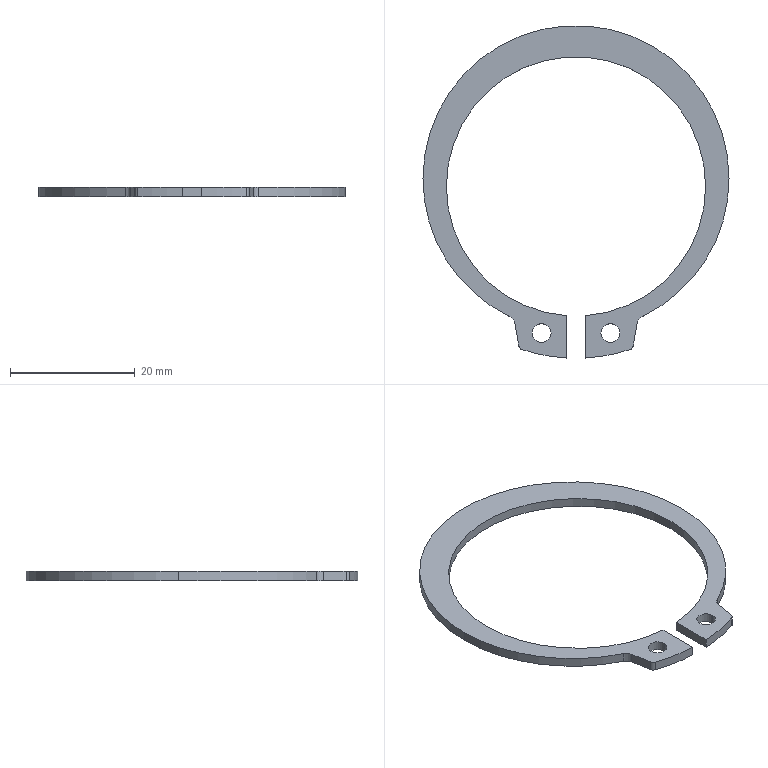Part | SolidWorks | features BaseBody 1 | 1 solid | 22 faces | box 49 x 53.209 x 1.5 mm | volume 871.359 mm3 | cylinder 16 | plane 6 | commonest cylinder face diameters 3 x6 41.5 x3 49 x3 1.4 x2 55 x2
STEP:
#1=CARTESIAN_POINT('',(4.,-24.714,-1.5));
#2=VERTEX_POINT('',#1);
#3=CARTESIAN_POINT('',(7.,-24.714,-1.5));
#4=VERTEX_POINT('',#3);
#5=CARTESIAN_POINT('',(5.5,-24.714,-1.5));
#6=DIRECTION('',(0.,0.,1.));
#7=DIRECTION('',(-1.,0.,0.));
#8=AXIS2_PLACEMENT_3D('',#5,#6,#7);
#9=CIRCLE('',#8,1.5);
#10=EDGE_CURVE('',#2,#4,#9,.T.);
#11=ORIENTED_EDGE('',*,*,#10,.F.);
#12=CARTESIAN_POINT('',(4.,-24.714,0.));
#13=VERTEX_POINT('',#12);
#14=CARTESIAN_POINT('',(4.,-24.714,-1.5));
#15=DIRECTION('',(0.,0.,1.));
#16=VECTOR('',#15,1000.);
#17=LINE('',#14,#16);
#18=EDGE_CURVE('',#2,#13,#17,.T.);
#19=ORIENTED_EDGE('',*,*,#18,.T.);
#20=CARTESIAN_POINT('',(7.,-24.714,0.));
#21=VERTEX_POINT('',#20);
#22=CARTESIAN_POINT('',(5.5,-24.714,0.));
#23=DIRECTION('',(0.,0.,1.));
#24=DIRECTION('',(-1.,0.,0.));
#25=AXIS2_PLACEMENT_3D('',#22,#23,#24);
#26=CIRCLE('',#25,1.5);
#27=EDGE_CURVE('',#13,#21,#26,.T.);
#28=ORIENTED_EDGE('',*,*,#27,.T.);
#29=CARTESIAN_POINT('',(7.,-24.714,-1.5));
#30=DIRECTION('',(0.,0.,1.));
#31=VECTOR('',#30,1000.);
#32=LINE('',#29,#31);
#33=EDGE_CURVE('',#4,#21,#32,.T.);
#34=ORIENTED_EDGE('',*,*,#33,.F.);
#35=EDGE_LOOP('',(#11,#19,#28,#34));
#36=FACE_OUTER_BOUND('',#35,.T.);
#37=CARTESIAN_POINT('',(5.5,-24.714,-1.5));
#38=DIRECTION('',(0.,0.,1.));
#39=DIRECTION('',(1.,0.,0.));
#40=AXIS2_PLACEMENT_3D('',#37,#38,#39);
#41=CYLINDRICAL_SURFACE('',#40,1.5);
#42=ADVANCED_FACE('',(#36),#41,.F.);
#43=CARTESIAN_POINT('',(-7.,-24.714,-1.5));
#44=VERTEX_POINT('',#43);
#45=CARTESIAN_POINT('',(-4.,-24.714,-1.5));
#46=VERTEX_POINT('',#45);
#47=CARTESIAN_POINT('',(-5.5,-24.714,-1.5));
#48=DIRECTION('',(0.,0.,1.));
#49=DIRECTION('',(1.,0.,0.));
#50=AXIS2_PLACEMENT_3D('',#47,#48,#49);
#51=CIRCLE('',#50,1.5);
#52=EDGE_CURVE('',#44,#46,#51,.T.);
#53=ORIENTED_EDGE('',*,*,#52,.F.);
#54=CARTESIAN_POINT('',(-7.,-24.714,0.));
#55=VERTEX_POINT('',#54);
#56=CARTESIAN_POINT('',(-7.,-24.714,-1.5));
#57=DIRECTION('',(0.,0.,1.));
#58=VECTOR('',#57,1000.);
#59=LINE('',#56,#58);
#60=EDGE_CURVE('',#44,#55,#59,.T.);
#61=ORIENTED_EDGE('',*,*,#60,.T.);
#62=CARTESIAN_POINT('',(-4.,-24.714,0.));
#63=VERTEX_POINT('',#62);
#64=CARTESIAN_POINT('',(-5.5,-24.714,0.));
#65=DIRECTION('',(0.,0.,1.));
#66=DIRECTION('',(1.,0.,0.));
#67=AXIS2_PLACEMENT_3D('',#64,#65,#66);
#68=CIRCLE('',#67,1.5);
#69=EDGE_CURVE('',#55,#63,#68,.T.);
#70=ORIENTED_EDGE('',*,*,#69,.T.);
#71=CARTESIAN_POINT('',(-4.,-24.714,-1.5));
#72=DIRECTION('',(0.,0.,1.));
#73=VECTOR('',#72,1000.);
#74=LINE('',#71,#73);
#75=EDGE_CURVE('',#46,#63,#74,.T.);
#76=ORIENTED_EDGE('',*,*,#75,.F.);
#77=EDGE_LOOP('',(#53,#61,#70,#76));
#78=FACE_OUTER_BOUND('',#77,.T.);
#79=CARTESIAN_POINT('',(-5.5,-24.714,-1.5));
#80=DIRECTION('',(0.,0.,1.));
#81=DIRECTION('',(1.,0.,0.));
#82=AXIS2_PLACEMENT_3D('',#79,#80,#81);
#83=CYLINDRICAL_SURFACE('',#82,1.5);
#84=ADVANCED_FACE('',(#78),#83,.F.);
#85=CARTESIAN_POINT('',(24.5,0.,-1.5));
#86=VERTEX_POINT('',#85);
#87=CARTESIAN_POINT('',(-24.5,0.,-1.5));
#88=VERTEX_POINT('',#87);
#89=CARTESIAN_POINT('',(0.,0.,-1.5));
#90=DIRECTION('',(0.,0.,1.));
#91=DIRECTION('',(1.,0.,0.));
#92=AXIS2_PLACEMENT_3D('',#89,#90,#91);
#93=CIRCLE('',#92,24.5);
#94=EDGE_CURVE('',#86,#88,#93,.T.);
#95=ORIENTED_EDGE('',*,*,#94,.T.);
#96=CARTESIAN_POINT('',(-24.5,0.,0.));
#97=VERTEX_POINT('',#96);
#98=CARTESIAN_POINT('',(-24.5,0.,-1.5));
#99=DIRECTION('',(0.,0.,1.));
#100=VECTOR('',#99,1000.);
#101=LINE('',#98,#100);
#102=EDGE_CURVE('',#88,#97,#101,.T.);
#103=ORIENTED_EDGE('',*,*,#102,.T.);
#104=CARTESIAN_POINT('',(24.5,0.,0.));
#105=VERTEX_POINT('',#104);
#106=CARTESIAN_POINT('',(0.,0.,0.));
#107=DIRECTION('',(0.,0.,1.));
#108=DIRECTION('',(1.,0.,0.));
#109=AXIS2_PLACEMENT_3D('',#106,#107,#108);
#110=CIRCLE('',#109,24.5);
#111=EDGE_CURVE('',#105,#97,#110,.T.);
#112=ORIENTED_EDGE('',*,*,#111,.F.);
#113=CARTESIAN_POINT('',(24.5,0.,-1.5));
#114=DIRECTION('',(0.,0.,1.));
#115=VECTOR('',#114,1000.);
#116=LINE('',#113,#115);
#117=EDGE_CURVE('',#86,#105,#116,.T.);
#118=ORIENTED_EDGE('',*,*,#117,.F.);
#119=EDGE_LOOP('',(#95,#103,#112,#118));
#120=FACE_OUTER_BOUND('',#119,.T.);
#121=CARTESIAN_POINT('',(0.,0.,-1.5));
#122=DIRECTION('',(0.,0.,1.));
#123=DIRECTION('',(1.,0.,0.));
#124=AXIS2_PLACEMENT_3D('',#121,#122,#123);
#125=CYLINDRICAL_SURFACE('',#124,24.5);
#126=ADVANCED_FACE('',(#120),#125,.T.);
#127=CARTESIAN_POINT('',(10.615,-22.081,-1.5));
#128=VERTEX_POINT('',#127);
#129=CARTESIAN_POINT('',(0.,0.,-1.5));
#130=DIRECTION('',(0.,0.,1.));
#131=DIRECTION('',(1.,0.,0.));
#132=AXIS2_PLACEMENT_3D('',#129,#130,#131);
#133=CIRCLE('',#132,24.5);
#134=EDGE_CURVE('',#128,#86,#133,.T.);
#135=ORIENTED_EDGE('',*,*,#134,.T.);
#136=ORIENTED_EDGE('',*,*,#117,.T.);
#137=CARTESIAN_POINT('',(10.615,-22.081,0.));
#138=VERTEX_POINT('',#137);
#139=CARTESIAN_POINT('',(0.,0.,0.));
#140=DIRECTION('',(0.,0.,1.));
#141=DIRECTION('',(1.,0.,0.));
#142=AXIS2_PLACEMENT_3D('',#139,#140,#141);
#143=CIRCLE('',#142,24.5);
#144=EDGE_CURVE('',#138,#105,#143,.T.);
#145=ORIENTED_EDGE('',*,*,#144,.F.);
#146=CARTESIAN_POINT('',(10.615,-22.081,-1.5));
#147=DIRECTION('',(0.,0.,-1.));
#148=VECTOR('',#147,1000.);
#149=LINE('',#146,#148);
#150=EDGE_CURVE('',#138,#128,#149,.T.);
#151=ORIENTED_EDGE('',*,*,#150,.T.);
#152=EDGE_LOOP('',(#135,#136,#145,#151));
#153=FACE_OUTER_BOUND('',#152,.T.);
#154=CARTESIAN_POINT('',(0.,0.,-1.5));
#155=DIRECTION('',(0.,0.,1.));
#156=DIRECTION('',(1.,0.,0.));
#157=AXIS2_PLACEMENT_3D('',#154,#155,#156);
#158=CYLINDRICAL_SURFACE('',#157,24.5);
#159=ADVANCED_FACE('',(#153),#158,.T.);
#160=CARTESIAN_POINT('',(-1.5,-21.946,-1.5));
#161=VERTEX_POINT('',#160);
#162=CARTESIAN_POINT('',(-20.75,-1.25,-1.5));
#163=VERTEX_POINT('',#162);
#164=CARTESIAN_POINT('',(0.,-1.25,-1.5));
#165=DIRECTION('',(0.,0.,-1.));
#166=DIRECTION('',(1.,0.,0.));
#167=AXIS2_PLACEMENT_3D('',#164,#165,#166);
#168=CIRCLE('',#167,20.75);
#169=EDGE_CURVE('',#161,#163,#168,.T.);
#170=ORIENTED_EDGE('',*,*,#169,.T.);
#171=CARTESIAN_POINT('',(-20.75,-1.25,0.));
#172=VERTEX_POINT('',#171);
#173=CARTESIAN_POINT('',(-20.75,-1.25,-1.5));
#174=DIRECTION('',(0.,0.,1.));
#175=VECTOR('',#174,1000.);
#176=LINE('',#173,#175);
#177=EDGE_CURVE('',#163,#172,#176,.T.);
#178=ORIENTED_EDGE('',*,*,#177,.T.);
#179=CARTESIAN_POINT('',(-1.5,-21.946,0.));
#180=VERTEX_POINT('',#179);
#181=CARTESIAN_POINT('',(0.,-1.25,0.));
#182=DIRECTION('',(0.,0.,-1.));
#183=DIRECTION('',(1.,0.,0.));
#184=AXIS2_PLACEMENT_3D('',#181,#182,#183);
#185=CIRCLE('',#184,20.75);
#186=EDGE_CURVE('',#180,#172,#185,.T.);
#187=ORIENTED_EDGE('',*,*,#186,.F.);
#188=CARTESIAN_POINT('',(-1.5,-21.946,-1.5));
#189=DIRECTION('',(0.,0.,1.));
#190=VECTOR('',#189,1000.);
#191=LINE('',#188,#190);
#192=EDGE_CURVE('',#161,#180,#191,.T.);
#193=ORIENTED_EDGE('',*,*,#192,.F.);
#194=EDGE_LOOP('',(#170,#178,#187,#193));
#195=FACE_OUTER_BOUND('',#194,.T.);
#196=CARTESIAN_POINT('',(0.,-1.25,-1.5));
#197=DIRECTION('',(0.,0.,1.));
#198=DIRECTION('',(1.,0.,0.));
#199=AXIS2_PLACEMENT_3D('',#196,#197,#198);
#200=CYLINDRICAL_SURFACE('',#199,20.75);
#201=ADVANCED_FACE('',(#195),#200,.F.);
#202=ORIENTED_EDGE('',*,*,#177,.F.);
#203=CARTESIAN_POINT('',(20.75,-1.25,-1.5));
#204=VERTEX_POINT('',#203);
#205=CARTESIAN_POINT('',(0.,-1.25,-1.5));
#206=DIRECTION('',(0.,0.,-1.));
#207=DIRECTION('',(1.,0.,0.));
#208=AXIS2_PLACEMENT_3D('',#205,#206,#207);
#209=CIRCLE('',#208,20.75);
#210=EDGE_CURVE('',#163,#204,#209,.T.);
#211=ORIENTED_EDGE('',*,*,#210,.T.);
#212=CARTESIAN_POINT('',(20.75,-1.25,0.));
#213=VERTEX_POINT('',#212);
#214=CARTESIAN_POINT('',(20.75,-1.25,-1.5));
#215=DIRECTION('',(0.,0.,1.));
#216=VECTOR('',#215,1000.);
#217=LINE('',#214,#216);
#218=EDGE_CURVE('',#204,#213,#217,.T.);
#219=ORIENTED_EDGE('',*,*,#218,.T.);
#220=CARTESIAN_POINT('',(0.,-1.25,0.));
#221=DIRECTION('',(0.,0.,-1.));
#222=DIRECTION('',(1.,0.,0.));
#223=AXIS2_PLACEMENT_3D('',#220,#221,#222);
#224=CIRCLE('',#223,20.75);
#225=EDGE_CURVE('',#172,#213,#224,.T.);
#226=ORIENTED_EDGE('',*,*,#225,.F.);
#227=EDGE_LOOP('',(#202,#211,#219,#226));
#228=FACE_OUTER_BOUND('',#227,.T.);
#229=CARTESIAN_POINT('',(0.,-1.25,-1.5));
#230=DIRECTION('',(0.,0.,1.));
#231=DIRECTION('',(1.,0.,0.));
#232=AXIS2_PLACEMENT_3D('',#229,#230,#231);
#233=CYLINDRICAL_SURFACE('',#232,20.75);
#234=ADVANCED_FACE('',(#228),#233,.F.);
#235=CARTESIAN_POINT('',(1.5,-28.709,-1.5));
#236=VERTEX_POINT('',#235);
#237=CARTESIAN_POINT('',(8.679,-27.344,-1.5));
#238=VERTEX_POINT('',#237);
#239=CARTESIAN_POINT('',(0.,-1.25,-1.5));
#240=DIRECTION('',(0.,0.,1.));
#241=DIRECTION('',(-1.,0.,0.));
#242=AXIS2_PLACEMENT_3D('',#239,#240,#241);
#243=CIRCLE('',#242,27.5);
#244=EDGE_CURVE('',#236,#238,#243,.T.);
#245=ORIENTED_EDGE('',*,*,#244,.T.);
#246=CARTESIAN_POINT('',(8.679,-27.344,0.));
#247=VERTEX_POINT('',#246);
#248=CARTESIAN_POINT('',(8.679,-27.344,-1.5));
#249=DIRECTION('',(0.,0.,1.));
#250=VECTOR('',#249,1000.);
#251=LINE('',#248,#250);
#252=EDGE_CURVE('',#238,#247,#251,.T.);
#253=ORIENTED_EDGE('',*,*,#252,.T.);
#254=CARTESIAN_POINT('',(1.5,-28.709,0.));
#255=VERTEX_POINT('',#254);
#256=CARTESIAN_POINT('',(0.,-1.25,0.));
#257=DIRECTION('',(0.,0.,1.));
#258=DIRECTION('',(-1.,0.,0.));
#259=AXIS2_PLACEMENT_3D('',#256,#257,#258);
#260=CIRCLE('',#259,27.5);
#261=EDGE_CURVE('',#255,#247,#260,.T.);
#262=ORIENTED_EDGE('',*,*,#261,.F.);
#263=CARTESIAN_POINT('',(1.5,-28.709,-1.5));
#264=DIRECTION('',(0.,0.,1.));
#265=VECTOR('',#264,1000.);
#266=LINE('',#263,#265);
#267=EDGE_CURVE('',#236,#255,#266,.T.);
#268=ORIENTED_EDGE('',*,*,#267,.F.);
#269=EDGE_LOOP('',(#245,#253,#262,#268));
#270=FACE_OUTER_BOUND('',#269,.T.);
#271=CARTESIAN_POINT('',(0.,-1.25,-1.5));
#272=DIRECTION('',(0.,0.,1.));
#273=DIRECTION('',(1.,0.,0.));
#274=AXIS2_PLACEMENT_3D('',#271,#272,#273);
#275=CYLINDRICAL_SURFACE('',#274,27.5);
#276=ADVANCED_FACE('',(#270),#275,.T.);
#277=CARTESIAN_POINT('',(1.5,-21.946,0.));
#278=VERTEX_POINT('',#277);
#279=CARTESIAN_POINT('',(1.5,-21.946,0.));
#280=DIRECTION('',(0.,-1.,0.));
#281=VECTOR('',#280,1000.);
#282=LINE('',#279,#281);
#283=EDGE_CURVE('',#278,#255,#282,.T.);
#284=ORIENTED_EDGE('',*,*,#283,.F.);
#285=CARTESIAN_POINT('',(1.5,-21.946,-1.5));
#286=VERTEX_POINT('',#285);
#287=CARTESIAN_POINT('',(1.5,-21.946,-1.5));
#288=DIRECTION('',(0.,0.,1.));
#289=VECTOR('',#288,1000.);
#290=LINE('',#287,#289);
#291=EDGE_CURVE('',#286,#278,#290,.T.);
#292=ORIENTED_EDGE('',*,*,#291,.F.);
#293=CARTESIAN_POINT('',(1.5,-21.946,-1.5));
#294=DIRECTION('',(0.,-1.,0.));
#295=VECTOR('',#294,1000.);
#296=LINE('',#293,#295);
#297=EDGE_CURVE('',#286,#236,#296,.T.);
#298=ORIENTED_EDGE('',*,*,#297,.T.);
#299=ORIENTED_EDGE('',*,*,#267,.T.);
#300=EDGE_LOOP('',(#284,#292,#298,#299));
#301=FACE_OUTER_BOUND('',#300,.T.);
#302=CARTESIAN_POINT('',(1.5,-21.946,-1.5));
#303=DIRECTION('',(-1.,0.,0.));
#304=DIRECTION('',(0.,-1.,0.));
#305=AXIS2_PLACEMENT_3D('',#302,#303,#304);
#306=PLANE('',#305);
#307=ADVANCED_FACE('',(#301),#306,.T.);
#308=ORIENTED_EDGE('',*,*,#218,.F.);
#309=CARTESIAN_POINT('',(0.,-1.25,-1.5));
#310=DIRECTION('',(0.,0.,-1.));
#311=DIRECTION('',(1.,0.,0.));
#312=AXIS2_PLACEMENT_3D('',#309,#310,#311);
#313=CIRCLE('',#312,20.75);
#314=EDGE_CURVE('',#204,#286,#313,.T.);
#315=ORIENTED_EDGE('',*,*,#314,.T.);
#316=ORIENTED_EDGE('',*,*,#291,.T.);
#317=CARTESIAN_POINT('',(0.,-1.25,0.));
#318=DIRECTION('',(0.,0.,-1.));
#319=DIRECTION('',(1.,0.,0.));
#320=AXIS2_PLACEMENT_3D('',#317,#318,#319);
#321=CIRCLE('',#320,20.75);
#322=EDGE_CURVE('',#213,#278,#321,.T.);
#323=ORIENTED_EDGE('',*,*,#322,.F.);
#324=EDGE_LOOP('',(#308,#315,#316,#323));
#325=FACE_OUTER_BOUND('',#324,.T.);
#326=CARTESIAN_POINT('',(0.,-1.25,-1.5));
#327=DIRECTION('',(0.,0.,1.));
#328=DIRECTION('',(1.,0.,0.));
#329=AXIS2_PLACEMENT_3D('',#326,#327,#328);
#330=CYLINDRICAL_SURFACE('',#329,20.75);
#331=ADVANCED_FACE('',(#325),#330,.F.);
#332=CARTESIAN_POINT('',(-1.5,-28.709,0.));
#333=VERTEX_POINT('',#332);
#334=CARTESIAN_POINT('',(-1.5,-21.946,0.));
#335=DIRECTION('',(0.,1.,0.));
#336=VECTOR('',#335,1000.);
#337=LINE('',#334,#336);
#338=EDGE_CURVE('',#333,#180,#337,.T.);
#339=ORIENTED_EDGE('',*,*,#338,.F.);
#340=CARTESIAN_POINT('',(-1.5,-28.709,-1.5));
#341=VERTEX_POINT('',#340);
#342=CARTESIAN_POINT('',(-1.5,-28.709,-1.5));
#343=DIRECTION('',(0.,0.,1.));
#344=VECTOR('',#343,1000.);
#345=LINE('',#342,#344);
#346=EDGE_CURVE('',#341,#333,#345,.T.);
#347=ORIENTED_EDGE('',*,*,#346,.F.);
#348=CARTESIAN_POINT('',(-1.5,-21.946,-1.5));
#349=DIRECTION('',(0.,1.,0.));
#350=VECTOR('',#349,1000.);
#351=LINE('',#348,#350);
#352=EDGE_CURVE('',#341,#161,#351,.T.);
#353=ORIENTED_EDGE('',*,*,#352,.T.);
#354=ORIENTED_EDGE('',*,*,#192,.T.);
#355=EDGE_LOOP('',(#339,#347,#353,#354));
#356=FACE_OUTER_BOUND('',#355,.T.);
#357=CARTESIAN_POINT('',(-1.5,-21.946,-1.5));
#358=DIRECTION('',(1.,0.,0.));
#359=DIRECTION('',(0.,1.,0.));
#360=AXIS2_PLACEMENT_3D('',#357,#358,#359);
#361=PLANE('',#360);
#362=ADVANCED_FACE('',(#356),#361,.T.);
#363=CARTESIAN_POINT('',(-8.679,-27.344,0.));
#364=VERTEX_POINT('',#363);
#365=CARTESIAN_POINT('',(0.,-1.25,0.));
#366=DIRECTION('',(0.,0.,1.));
#367=DIRECTION('',(1.,0.,0.));
#368=AXIS2_PLACEMENT_3D('',#365,#366,#367);
#369=CIRCLE('',#368,27.5);
#370=EDGE_CURVE('',#364,#333,#369,.T.);
#371=ORIENTED_EDGE('',*,*,#370,.F.);
#372=CARTESIAN_POINT('',(-8.679,-27.344,-1.5));
#373=VERTEX_POINT('',#372);
#374=CARTESIAN_POINT('',(-8.679,-27.344,-1.5));
#375=DIRECTION('',(0.,0.,-1.));
#376=VECTOR('',#375,1000.);
#377=LINE('',#374,#376);
#378=EDGE_CURVE('',#364,#373,#377,.T.);
#379=ORIENTED_EDGE('',*,*,#378,.T.);
#380=CARTESIAN_POINT('',(0.,-1.25,-1.5));
#381=DIRECTION('',(0.,0.,1.));
#382=DIRECTION('',(1.,0.,0.));
#383=AXIS2_PLACEMENT_3D('',#380,#381,#382);
#384=CIRCLE('',#383,27.5);
#385=EDGE_CURVE('',#373,#341,#384,.T.);
#386=ORIENTED_EDGE('',*,*,#385,.T.);
#387=ORIENTED_EDGE('',*,*,#346,.T.);
#388=EDGE_LOOP('',(#371,#379,#386,#387));
#389=FACE_OUTER_BOUND('',#388,.T.);
#390=CARTESIAN_POINT('',(0.,-1.25,-1.5));
#391=DIRECTION('',(0.,0.,1.));
#392=DIRECTION('',(1.,0.,0.));
#393=AXIS2_PLACEMENT_3D('',#390,#391,#392);
#394=CYLINDRICAL_SURFACE('',#393,27.5);
#395=ADVANCED_FACE('',(#389),#394,.T.);
#396=CARTESIAN_POINT('',(-9.788,-23.172,0.));
#397=VERTEX_POINT('',#396);
#398=CARTESIAN_POINT('',(-9.148,-26.802,0.));
#399=VERTEX_POINT('',#398);
#400=CARTESIAN_POINT('',(-9.924,-22.4,0.));
#401=DIRECTION('',(0.1736,-0.9848,0.));
#402=VECTOR('',#401,1000.);
#403=LINE('',#400,#402);
#404=EDGE_CURVE('',#397,#399,#403,.T.);
#405=ORIENTED_EDGE('',*,*,#404,.F.);
#406=CARTESIAN_POINT('',(-9.788,-23.172,-1.5));
#407=VERTEX_POINT('',#406);
#408=CARTESIAN_POINT('',(-9.788,-23.172,-1.5));
#409=DIRECTION('',(0.,0.,-1.));
#410=VECTOR('',#409,1000.);
#411=LINE('',#408,#410);
#412=EDGE_CURVE('',#397,#407,#411,.T.);
#413=ORIENTED_EDGE('',*,*,#412,.T.);
#414=CARTESIAN_POINT('',(-9.148,-26.802,-1.5));
#415=VERTEX_POINT('',#414);
#416=CARTESIAN_POINT('',(-9.924,-22.4,-1.5));
#417=DIRECTION('',(0.1736,-0.9848,0.));
#418=VECTOR('',#417,1000.);
#419=LINE('',#416,#418);
#420=EDGE_CURVE('',#407,#415,#419,.T.);
#421=ORIENTED_EDGE('',*,*,#420,.T.);
#422=CARTESIAN_POINT('',(-9.148,-26.802,-1.5));
#423=DIRECTION('',(0.,0.,1.));
#424=VECTOR('',#423,1000.);
#425=LINE('',#422,#424);
#426=EDGE_CURVE('',#415,#399,#425,.T.);
#427=ORIENTED_EDGE('',*,*,#426,.T.);
#428=EDGE_LOOP('',(#405,#413,#421,#427));
#429=FACE_OUTER_BOUND('',#428,.T.);
#430=CARTESIAN_POINT('',(-9.924,-22.4,-1.5));
#431=DIRECTION('',(-0.9848,-0.1736,0.));
#432=DIRECTION('',(0.1736,-0.9848,0.));
#433=AXIS2_PLACEMENT_3D('',#430,#431,#432);
#434=PLANE('',#433);
#435=ADVANCED_FACE('',(#429),#434,.T.);
#436=ORIENTED_EDGE('',*,*,#102,.F.);
#437=CARTESIAN_POINT('',(-10.615,-22.081,-1.5));
#438=VERTEX_POINT('',#437);
#439=CARTESIAN_POINT('',(0.,0.,-1.5));
#440=DIRECTION('',(0.,0.,1.));
#441=DIRECTION('',(1.,0.,0.));
#442=AXIS2_PLACEMENT_3D('',#439,#440,#441);
#443=CIRCLE('',#442,24.5);
#444=EDGE_CURVE('',#88,#438,#443,.T.);
#445=ORIENTED_EDGE('',*,*,#444,.T.);
#446=CARTESIAN_POINT('',(-10.615,-22.081,0.));
#447=VERTEX_POINT('',#446);
#448=CARTESIAN_POINT('',(-10.615,-22.081,-1.5));
#449=DIRECTION('',(0.,0.,1.));
#450=VECTOR('',#449,1000.);
#451=LINE('',#448,#450);
#452=EDGE_CURVE('',#438,#447,#451,.T.);
#453=ORIENTED_EDGE('',*,*,#452,.T.);
#454=CARTESIAN_POINT('',(0.,0.,0.));
#455=DIRECTION('',(0.,0.,1.));
#456=DIRECTION('',(1.,0.,0.));
#457=AXIS2_PLACEMENT_3D('',#454,#455,#456);
#458=CIRCLE('',#457,24.5);
#459=EDGE_CURVE('',#97,#447,#458,.T.);
#460=ORIENTED_EDGE('',*,*,#459,.F.);
#461=EDGE_LOOP('',(#436,#445,#453,#460));
#462=FACE_OUTER_BOUND('',#461,.T.);
#463=CARTESIAN_POINT('',(0.,0.,-1.5));
#464=DIRECTION('',(0.,0.,1.));
#465=DIRECTION('',(1.,0.,0.));
#466=AXIS2_PLACEMENT_3D('',#463,#464,#465);
#467=CYLINDRICAL_SURFACE('',#466,24.5);
#468=ADVANCED_FACE('',(#462),#467,.T.);
#469=CARTESIAN_POINT('',(9.148,-26.802,-1.5));
#470=VERTEX_POINT('',#469);
#471=CARTESIAN_POINT('',(9.788,-23.172,-1.5));
#472=VERTEX_POINT('',#471);
#473=CARTESIAN_POINT('',(9.924,-22.4,-1.5));
#474=DIRECTION('',(0.1736,0.9848,0.));
#475=VECTOR('',#474,1000.);
#476=LINE('',#473,#475);
#477=EDGE_CURVE('',#470,#472,#476,.T.);
#478=ORIENTED_EDGE('',*,*,#477,.T.);
#479=CARTESIAN_POINT('',(9.788,-23.172,0.));
#480=VERTEX_POINT('',#479);
#481=CARTESIAN_POINT('',(9.788,-23.172,0.));
#482=DIRECTION('',(0.,0.,1.));
#483=VECTOR('',#482,1000.);
#484=LINE('',#481,#483);
#485=EDGE_CURVE('',#472,#480,#484,.T.);
#486=ORIENTED_EDGE('',*,*,#485,.T.);
#487=CARTESIAN_POINT('',(9.148,-26.802,0.));
#488=VERTEX_POINT('',#487);
#489=CARTESIAN_POINT('',(9.924,-22.4,0.));
#490=DIRECTION('',(0.1736,0.9848,0.));
#491=VECTOR('',#490,1000.);
#492=LINE('',#489,#491);
#493=EDGE_CURVE('',#488,#480,#492,.T.);
#494=ORIENTED_EDGE('',*,*,#493,.F.);
#495=CARTESIAN_POINT('',(9.148,-26.802,-1.5));
#496=DIRECTION('',(0.,0.,-1.));
#497=VECTOR('',#496,1000.);
#498=LINE('',#495,#497);
#499=EDGE_CURVE('',#488,#470,#498,.T.);
#500=ORIENTED_EDGE('',*,*,#499,.T.);
#501=EDGE_LOOP('',(#478,#486,#494,#500));
#502=FACE_OUTER_BOUND('',#501,.T.);
#503=CARTESIAN_POINT('',(9.924,-22.4,-1.5));
#504=DIRECTION('',(0.9848,-0.1736,0.));
#505=DIRECTION('',(0.1736,0.9848,0.));
#506=AXIS2_PLACEMENT_3D('',#503,#504,#505);
#507=PLANE('',#506);
#508=ADVANCED_FACE('',(#502),#507,.T.);
#509=CARTESIAN_POINT('',(5.5,-24.714,-1.5));
#510=DIRECTION('',(0.,0.,1.));
#511=DIRECTION('',(-1.,0.,0.));
#512=AXIS2_PLACEMENT_3D('',#509,#510,#511);
#513=CIRCLE('',#512,1.5);
#514=EDGE_CURVE('',#4,#2,#513,.T.);
#515=ORIENTED_EDGE('',*,*,#514,.T.);
#516=ORIENTED_EDGE('',*,*,#10,.T.);
#517=EDGE_LOOP('',(#515,#516));
#518=FACE_BOUND('',#517,.T.);
#519=CARTESIAN_POINT('',(-5.5,-24.714,-1.5));
#520=DIRECTION('',(0.,0.,1.));
#521=DIRECTION('',(1.,0.,0.));
#522=AXIS2_PLACEMENT_3D('',#519,#520,#521);
#523=CIRCLE('',#522,1.5);
#524=EDGE_CURVE('',#46,#44,#523,.T.);
#525=ORIENTED_EDGE('',*,*,#524,.T.);
#526=ORIENTED_EDGE('',*,*,#52,.T.);
#527=EDGE_LOOP('',(#525,#526));
#528=FACE_BOUND('',#527,.T.);
#529=ORIENTED_EDGE('',*,*,#385,.F.);
#530=CARTESIAN_POINT('',(-8.458,-26.68,-1.5));
#531=DIRECTION('',(0.,0.,-1.));
#532=DIRECTION('',(-1.,0.,0.));
#533=AXIS2_PLACEMENT_3D('',#530,#531,#532);
#534=CIRCLE('',#533,0.7);
#535=EDGE_CURVE('',#373,#415,#534,.T.);
#536=ORIENTED_EDGE('',*,*,#535,.T.);
#537=ORIENTED_EDGE('',*,*,#420,.F.);
#538=CARTESIAN_POINT('',(-11.265,-23.433,-1.5));
#539=DIRECTION('',(0.,0.,1.));
#540=DIRECTION('',(-1.,0.,0.));
#541=AXIS2_PLACEMENT_3D('',#538,#539,#540);
#542=CIRCLE('',#541,1.5);
#543=EDGE_CURVE('',#407,#438,#542,.T.);
#544=ORIENTED_EDGE('',*,*,#543,.T.);
#545=ORIENTED_EDGE('',*,*,#444,.F.);
#546=ORIENTED_EDGE('',*,*,#94,.F.);
#547=ORIENTED_EDGE('',*,*,#134,.F.);
#548=CARTESIAN_POINT('',(11.265,-23.433,-1.5));
#549=DIRECTION('',(0.,0.,1.));
#550=DIRECTION('',(-1.,0.,0.));
#551=AXIS2_PLACEMENT_3D('',#548,#549,#550);
#552=CIRCLE('',#551,1.5);
#553=EDGE_CURVE('',#128,#472,#552,.T.);
#554=ORIENTED_EDGE('',*,*,#553,.T.);
#555=ORIENTED_EDGE('',*,*,#477,.F.);
#556=CARTESIAN_POINT('',(8.458,-26.68,-1.5));
#557=DIRECTION('',(0.,0.,-1.));
#558=DIRECTION('',(-1.,0.,0.));
#559=AXIS2_PLACEMENT_3D('',#556,#557,#558);
#560=CIRCLE('',#559,0.7);
#561=EDGE_CURVE('',#470,#238,#560,.T.);
#562=ORIENTED_EDGE('',*,*,#561,.T.);
#563=ORIENTED_EDGE('',*,*,#244,.F.);
#564=ORIENTED_EDGE('',*,*,#297,.F.);
#565=ORIENTED_EDGE('',*,*,#314,.F.);
#566=ORIENTED_EDGE('',*,*,#210,.F.);
#567=ORIENTED_EDGE('',*,*,#169,.F.);
#568=ORIENTED_EDGE('',*,*,#352,.F.);
#569=EDGE_LOOP('',(#529,#536,#537,#544,#545,#546,#547,#554,#555,#562,#563,#564,#565,#566,#567,#568));
#570=FACE_OUTER_BOUND('',#569,.T.);
#571=CARTESIAN_POINT('',(0.,-1.25,-1.5));
#572=DIRECTION('',(0.,0.,-1.));
#573=DIRECTION('',(-1.,0.,0.));
#574=AXIS2_PLACEMENT_3D('',#571,#572,#573);
#575=PLANE('',#574);
#576=ADVANCED_FACE('',(#518,#528,#570),#575,.T.);
#577=CARTESIAN_POINT('',(5.5,-24.714,0.));
#578=DIRECTION('',(0.,0.,1.));
#579=DIRECTION('',(-1.,0.,0.));
#580=AXIS2_PLACEMENT_3D('',#577,#578,#579);
#581=CIRCLE('',#580,1.5);
#582=EDGE_CURVE('',#21,#13,#581,.T.);
#583=ORIENTED_EDGE('',*,*,#582,.F.);
#584=ORIENTED_EDGE('',*,*,#27,.F.);
#585=EDGE_LOOP('',(#583,#584));
#586=FACE_BOUND('',#585,.T.);
#587=CARTESIAN_POINT('',(-5.5,-24.714,0.));
#588=DIRECTION('',(0.,0.,1.));
#589=DIRECTION('',(1.,0.,0.));
#590=AXIS2_PLACEMENT_3D('',#587,#588,#589);
#591=CIRCLE('',#590,1.5);
#592=EDGE_CURVE('',#63,#55,#591,.T.);
#593=ORIENTED_EDGE('',*,*,#592,.F.);
#594=ORIENTED_EDGE('',*,*,#69,.F.);
#595=EDGE_LOOP('',(#593,#594));
#596=FACE_BOUND('',#595,.T.);
#597=ORIENTED_EDGE('',*,*,#144,.T.);
#598=ORIENTED_EDGE('',*,*,#111,.T.);
#599=ORIENTED_EDGE('',*,*,#459,.T.);
#600=CARTESIAN_POINT('',(-11.265,-23.433,0.));
#601=DIRECTION('',(0.,0.,-1.));
#602=DIRECTION('',(-1.,0.,0.));
#603=AXIS2_PLACEMENT_3D('',#600,#601,#602);
#604=CIRCLE('',#603,1.5);
#605=EDGE_CURVE('',#447,#397,#604,.T.);
#606=ORIENTED_EDGE('',*,*,#605,.T.);
#607=ORIENTED_EDGE('',*,*,#404,.T.);
#608=CARTESIAN_POINT('',(-8.458,-26.68,0.));
#609=DIRECTION('',(0.,0.,1.));
#610=DIRECTION('',(-1.,0.,0.));
#611=AXIS2_PLACEMENT_3D('',#608,#609,#610);
#612=CIRCLE('',#611,0.7);
#613=EDGE_CURVE('',#399,#364,#612,.T.);
#614=ORIENTED_EDGE('',*,*,#613,.T.);
#615=ORIENTED_EDGE('',*,*,#370,.T.);
#616=ORIENTED_EDGE('',*,*,#338,.T.);
#617=ORIENTED_EDGE('',*,*,#186,.T.);
#618=ORIENTED_EDGE('',*,*,#225,.T.);
#619=ORIENTED_EDGE('',*,*,#322,.T.);
#620=ORIENTED_EDGE('',*,*,#283,.T.);
#621=ORIENTED_EDGE('',*,*,#261,.T.);
#622=CARTESIAN_POINT('',(8.458,-26.68,0.));
#623=DIRECTION('',(0.,0.,1.));
#624=DIRECTION('',(-1.,0.,0.));
#625=AXIS2_PLACEMENT_3D('',#622,#623,#624);
#626=CIRCLE('',#625,0.7);
#627=EDGE_CURVE('',#247,#488,#626,.T.);
#628=ORIENTED_EDGE('',*,*,#627,.T.);
#629=ORIENTED_EDGE('',*,*,#493,.T.);
#630=CARTESIAN_POINT('',(11.265,-23.433,0.));
#631=DIRECTION('',(0.,0.,-1.));
#632=DIRECTION('',(-1.,0.,0.));
#633=AXIS2_PLACEMENT_3D('',#630,#631,#632);
#634=CIRCLE('',#633,1.5);
#635=EDGE_CURVE('',#480,#138,#634,.T.);
#636=ORIENTED_EDGE('',*,*,#635,.T.);
#637=EDGE_LOOP('',(#597,#598,#599,#606,#607,#614,#615,#616,#617,#618,#619,#620,#621,#628,#629,#636));
#638=FACE_OUTER_BOUND('',#637,.T.);
#639=CARTESIAN_POINT('',(0.,-1.25,0.));
#640=DIRECTION('',(0.,0.,-1.));
#641=DIRECTION('',(-1.,0.,0.));
#642=AXIS2_PLACEMENT_3D('',#639,#640,#641);
#643=PLANE('',#642);
#644=ADVANCED_FACE('',(#586,#596,#638),#643,.F.);
#645=ORIENTED_EDGE('',*,*,#60,.F.);
#646=ORIENTED_EDGE('',*,*,#524,.F.);
#647=ORIENTED_EDGE('',*,*,#75,.T.);
#648=ORIENTED_EDGE('',*,*,#592,.T.);
#649=EDGE_LOOP('',(#645,#646,#647,#648));
#650=FACE_OUTER_BOUND('',#649,.T.);
#651=CARTESIAN_POINT('',(-5.5,-24.714,-1.5));
#652=DIRECTION('',(0.,0.,1.));
#653=DIRECTION('',(1.,0.,0.));
#654=AXIS2_PLACEMENT_3D('',#651,#652,#653);
#655=CYLINDRICAL_SURFACE('',#654,1.5);
#656=ADVANCED_FACE('',(#650),#655,.F.);
#657=ORIENTED_EDGE('',*,*,#18,.F.);
#658=ORIENTED_EDGE('',*,*,#514,.F.);
#659=ORIENTED_EDGE('',*,*,#33,.T.);
#660=ORIENTED_EDGE('',*,*,#582,.T.);
#661=EDGE_LOOP('',(#657,#658,#659,#660));
#662=FACE_OUTER_BOUND('',#661,.T.);
#663=CARTESIAN_POINT('',(5.5,-24.714,-1.5));
#664=DIRECTION('',(0.,0.,1.));
#665=DIRECTION('',(1.,0.,0.));
#666=AXIS2_PLACEMENT_3D('',#663,#664,#665);
#667=CYLINDRICAL_SURFACE('',#666,1.5);
#668=ADVANCED_FACE('',(#662),#667,.F.);
#669=ORIENTED_EDGE('',*,*,#535,.F.);
#670=ORIENTED_EDGE('',*,*,#378,.F.);
#671=ORIENTED_EDGE('',*,*,#613,.F.);
#672=ORIENTED_EDGE('',*,*,#426,.F.);
#673=EDGE_LOOP('',(#669,#670,#671,#672));
#674=FACE_OUTER_BOUND('',#673,.T.);
#675=CARTESIAN_POINT('',(-8.458,-26.68,-1.5));
#676=DIRECTION('',(0.,0.,1.));
#677=DIRECTION('',(1.,0.,0.));
#678=AXIS2_PLACEMENT_3D('',#675,#676,#677);
#679=CYLINDRICAL_SURFACE('',#678,0.7);
#680=ADVANCED_FACE('',(#674),#679,.T.);
#681=ORIENTED_EDGE('',*,*,#561,.F.);
#682=ORIENTED_EDGE('',*,*,#499,.F.);
#683=ORIENTED_EDGE('',*,*,#627,.F.);
#684=ORIENTED_EDGE('',*,*,#252,.F.);
#685=EDGE_LOOP('',(#681,#682,#683,#684));
#686=FACE_OUTER_BOUND('',#685,.T.);
#687=CARTESIAN_POINT('',(8.458,-26.68,-1.5));
#688=DIRECTION('',(0.,0.,1.));
#689=DIRECTION('',(1.,0.,0.));
#690=AXIS2_PLACEMENT_3D('',#687,#688,#689);
#691=CYLINDRICAL_SURFACE('',#690,0.7);
#692=ADVANCED_FACE('',(#686),#691,.T.);
#693=ORIENTED_EDGE('',*,*,#553,.F.);
#694=ORIENTED_EDGE('',*,*,#150,.F.);
#695=ORIENTED_EDGE('',*,*,#635,.F.);
#696=ORIENTED_EDGE('',*,*,#485,.F.);
#697=EDGE_LOOP('',(#693,#694,#695,#696));
#698=FACE_OUTER_BOUND('',#697,.T.);
#699=CARTESIAN_POINT('',(11.265,-23.433,-1.5));
#700=DIRECTION('',(0.,0.,1.));
#701=DIRECTION('',(1.,0.,0.));
#702=AXIS2_PLACEMENT_3D('',#699,#700,#701);
#703=CYLINDRICAL_SURFACE('',#702,1.5);
#704=ADVANCED_FACE('',(#698),#703,.F.);
#705=ORIENTED_EDGE('',*,*,#543,.F.);
#706=ORIENTED_EDGE('',*,*,#412,.F.);
#707=ORIENTED_EDGE('',*,*,#605,.F.);
#708=ORIENTED_EDGE('',*,*,#452,.F.);
#709=EDGE_LOOP('',(#705,#706,#707,#708));
#710=FACE_OUTER_BOUND('',#709,.T.);
#711=CARTESIAN_POINT('',(-11.265,-23.433,-1.5));
#712=DIRECTION('',(0.,0.,1.));
#713=DIRECTION('',(1.,0.,0.));
#714=AXIS2_PLACEMENT_3D('',#711,#712,#713);
#715=CYLINDRICAL_SURFACE('',#714,1.5);
#716=ADVANCED_FACE('',(#710),#715,.F.);
#717=CLOSED_SHELL('',(#42,#84,#126,#159,#201,#234,#276,#307,#331,#362,#395,#435,#468,#508,#576,#644,#656,#668,#680,#692,#704,#716));
#718=MANIFOLD_SOLID_BREP('',#717);
#719=CARTESIAN_POINT('',(0.,0.,0.));
#720=DIRECTION('',(0.,0.,1.));
#721=DIRECTION('',(1.,0.,0.));
#722=AXIS2_PLACEMENT_3D('',#719,#720,#721);
#723=(LENGTH_UNIT()NAMED_UNIT(*)SI_UNIT(.MILLI.,.METRE.));
#724=UNCERTAINTY_MEASURE_WITH_UNIT(LENGTH_MEASURE(0.00001),#723,'','');
#725=(NAMED_UNIT(*)PLANE_ANGLE_UNIT()SI_UNIT($,.RADIAN.));
#726=(NAMED_UNIT(*)SI_UNIT($,.STERADIAN.)SOLID_ANGLE_UNIT());
#727=(GEOMETRIC_REPRESENTATION_CONTEXT(3)GLOBAL_UNCERTAINTY_ASSIGNED_CONTEXT((#724))GLOBAL_UNIT_ASSIGNED_CONTEXT((#723,#725,#726))REPRESENTATION_CONTEXT('',''));
#728=ADVANCED_BREP_SHAPE_REPRESENTATION('',(#718,#722),#727);